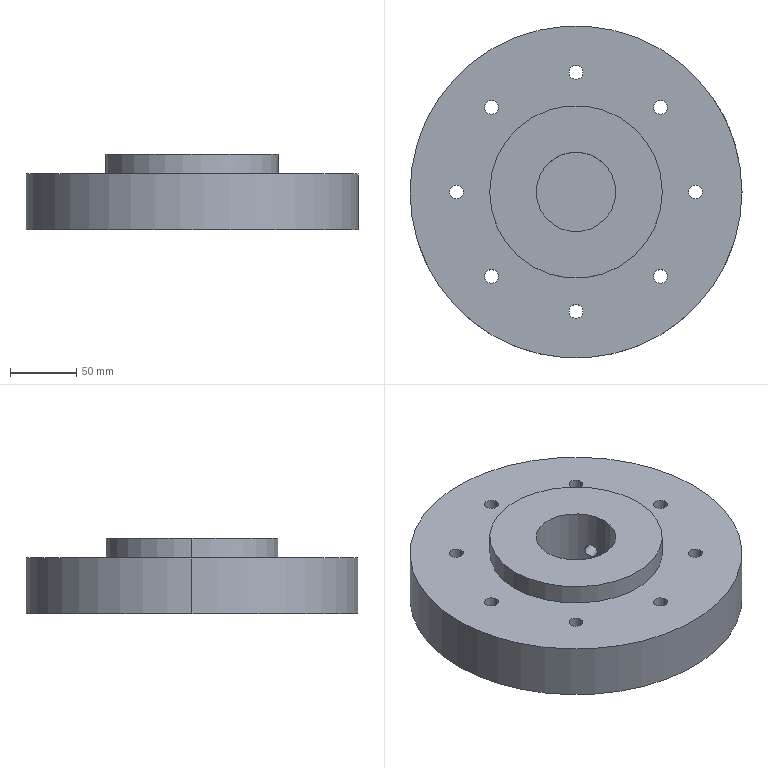Part | SolidWorks | features ICE 4, Extrusion 1, RevCut 1 | 1 solid | 61 faces | box 250 x 250 x 57.13 mm | volume 2053671 mm3 | cylinder 46 | plane 13 | cone 2 | commonest cylinder face diameters 10.5 x16 18 x16 10 x8 60 x2 130 x2 250 x2